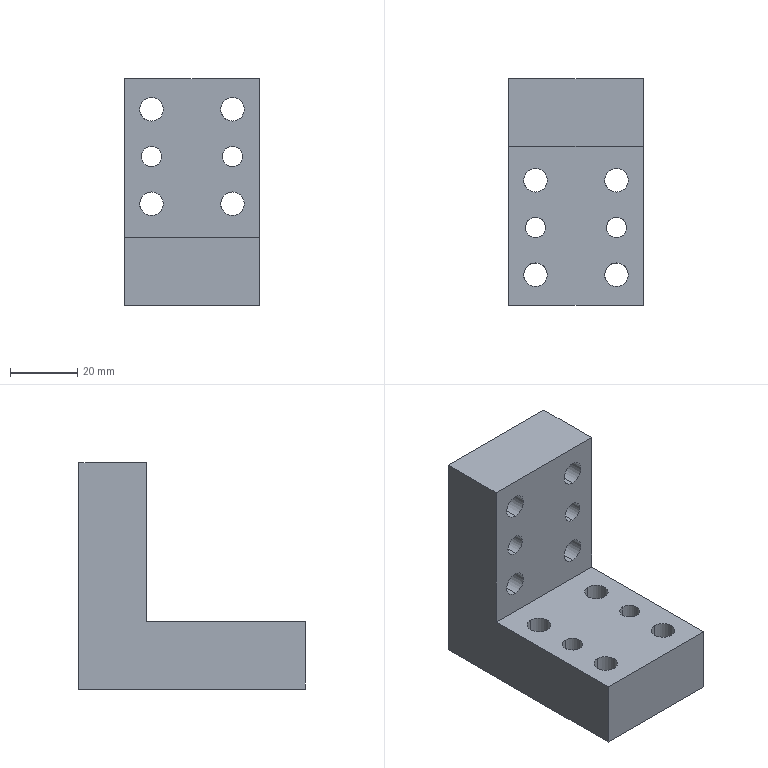Part | STEP file | Positioning_id2206_x_t | 1 solid | 32 faces | box 40 x 67 x 67 mm | volume 82781 mm3 | cylinder 24 | plane 8 | commonest cylinder face diameters 7 x16 6 x8